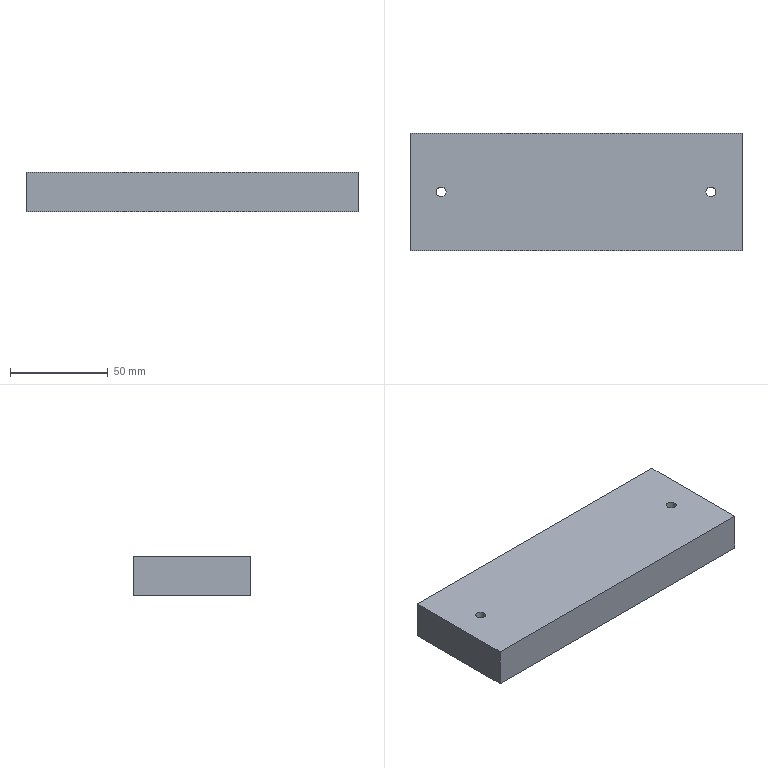CAM job | NX | 3-axis milling, drilling | part box 170 x 60 x 20 mm
Tools:
number,name,description,diameter,corner_radius,flute_length,length,flutes
15,D63,Milling Tool-5 Parameters,63.0,0.0,20.0,20.0,2
10,D12C,Milling Tool-5 Parameters,12.0,0.0,30.0,60.0,2
2,D8,Milling Tool-5 Parameters,8.0,0.0,20.0,50.0,2
3,D6,Milling Tool-5 Parameters,6.0,0.0,15.0,30.0,2
11,D6F,Milling Tool-5 Parameters,6.0,0.0,15.0,30.0,2
4,D4,Milling Tool-5 Parameters,4.0,0.0,10.0,30.0,2
12,D4F,Milling Tool-5 Parameters,4.0,0.0,10.0,25.0,2
5,D3,Milling Tool-5 Parameters,3.0,0.0,10.0,25.0,2
13,D3F,Milling Tool-5 Parameters,3.0,0.0,10.0,25.0,2
6,D2,Milling Tool-5 Parameters,2.0,0.0,5.0,10.0,2
7,D1,Milling Tool-5 Parameters,1.0,0.0,3.0,5.0,2
7,D4R0.5,Milling Tool-5 Parameters,4.0,0.5,10.0,30.0,2
7,D3R0.5,Milling Tool-5 Parameters,3.0,0.5,10.0,30.0,2
20,R1,Milling Tool-Ball Mill,2.0,1.0,5.0,10.0,2
9,D4V45,Milling Tool-5 Parameters,4.0,0.0,10.0,30.0,2
9,D6V45,Milling Tool-5 Parameters,6.0,0.0,10.0,30.0,2
18,ZD5.2,Drilling Tool,5.2,0.0,30.0,50.0,2
19,ZD5,Drilling Tool,5.0,0.0,30.0,35.0,2
12,ZD4.2,Drilling Tool,4.2,0.0,30.0,50.0,2
13,ZD3.3,Drilling Tool,3.3,0.0,30.0,50.0,2
21,ZD3,Drilling Tool,3.0,0.0,30.0,50.0,2
20,ZD1.2,Drilling Tool,1.2,0.0,30.0,50.0,2
20,D4.8-M6X1,Thread Mill,4.8,0.0,0.1,15.0,1
23,CT6,Centerdrill,6.0,0.0,0.0,50.0,2
Operations:
program,operation,operation_type,tool,method,geometry_group,spindle_rpm,surface_speed,feed_per_tooth,feed_cut,feed_plunge,cut_length_mm,path_length_mm,cut_time_min,machine_time_min
GP3-1-1,SPOT_DRILL._COPY,Operation,CT6,METHOD,W-1,3000.0,56.0,0.1667,1000.0,80.0,15.0,248.278,0.015,0.0383
GP3-1-1,DRILL._COPY,Operation,ZD5.2,METHOD,W-1,800.0,13.0,0.0625,100.0,80.0,49.124,257.253,0.4912,0.5121
GP3-1-1,DRILL._COPY_COPY,Operation,ZD3,METHOD,W-1,800.0,13.0,0.0625,100.0,80.0,24.0,202.472,0.24,0.2578
GP3-1-1,ZLEVEL_ROUGH._COPY,ZLevelMilling,D3,METHOD,W-1,5000.0,47.0,0.2,2000.0,80.0,623.78,850.615,0.3157,0.3383
GP3-1-1,ZLEVEL_FINISH._COPY,ZLevelMilling,D3R0.5,METHOD,W-1,8000.0,251.0,0.1875,3000.0,80.0,1064.424,1331.397,0.3554,0.3962
GP3-1-1,2D_CHAMFER._COPY,PlanarMilling,D6V45,METHOD,W-1,5000.0,125.0,0.1,1000.0,50.0,468.51,491.51,0.4701,0.4724
GP3-1-1,2D_CHAMFER._COPY_COPY,PlanarMilling,D6V45,METHOD,W-1,5000.0,125.0,0.1,1000.0,50.0,57.322,240.822,0.0635,0.0818
GP3-1-1,THREAD_MILL._COPY,ThreadMilling,D4.8-M6X1,METHOD,W-1,6000.0,90.0,0.3333,2000.0,50.0,241.604,519.604,0.1227,0.1505
GP3-1-2,3D_ROUGH_COPY,CavityMilling,D12C,METHOD,W-2,8000.0,301.0,0.375,6000.0,80.0,684.95,1013.851,0.1171,0.1657
GP3-1-2,ADAPTIVE_MILL_COPY,CavityMilling,D12C,METHOD,W-2,8000.0,301.0,0.25,4000.0,80.0,1559.391,1648.345,0.39,0.3989
GP3-1-2,3D_ROUGH_COPY_1,CavityMilling,D12C,METHOD,W-2,8000.0,301.0,0.375,6000.0,80.0,5873.405,7165.659,1.003,1.153
GP3-1-2,SPOT_DRILL_COPY,Operation,D6V45,METHOD,W-2,3000.0,56.0,0.25,1500.0,80.0,16.0,152.352,0.0107,0.0243
GP3-1-2,SPOT_DRILL_COPY_COPY,Operation,D6V45,METHOD,W-2,3000.0,56.0,0.25,1500.0,80.0,12.0,307.477,0.008,0.0375
GP3-1-2,SPOT_DRILL_COPY_COPY_COPY,Operation,D6V45,METHOD,W-2,3000.0,56.0,0.25,1500.0,80.0,8.0,131.034,0.0053,0.0176
GP3-1-2,DRILL_COPY,Operation,ZD5,METHOD,W-2,2000.0,32.0,0.075,300.0,80.0,45.004,182.968,0.15,0.1638
GP3-1-2,DRILL_COPY_COPY,Operation,ZD4.2,METHOD,W-2,2000.0,32.0,0.075,300.0,80.0,44.524,148.022,0.1484,0.1588
GP3-1-2,DRILL_COPY_1,Operation,ZD3.3,METHOD,W-2,2000.0,32.0,0.075,300.0,80.0,42.4,323.329,0.1413,0.1694
GP3-1-2,DRILL_COPY_1_COPY_1,Operation,ZD3.3,METHOD,W-2,2000.0,32.0,0.075,300.0,80.0,16.8,141.599,0.056,0.0685
GP3-1-2,DRILL_COPY_1_COPY,Operation,ZD1.2,METHOD,W-2,2000.0,7.0,0.025,100.0,80.0,120.484,361.32,1.205,1.229
GP3-1-2,3D_ROUGH_COPY_1_COPY,CavityMilling,D6,METHOD,W-2,10000.0,188.0,0.25,5000.0,80.0,4024.878,6570.952,0.8573,1.196
GP3-1-2,2D_LAYER_FINISH_MIDENTRY_COPY,PlanarMilling,D6,METHOD,W-2,10000.0,314.0,0.15,3000.0,50.0,199.534,676.857,0.0691,0.13
GP3-1-2,2D_HYBRID_MILL_COPY,PlanarMilling,D6,METHOD,W-2,10000.0,314.0,0.25,5000.0,80.0,991.46,1193.643,0.2003,0.2265
GP3-1-2,HOLE_MILL_COPY,CylinderMilling,D6,METHOD,W-2,10000.0,251.0,0.25,5000.0,80.0,372.596,612.336,0.0753,0.1029
GP3-1-2,2D_PLANAR_FINISH_COPY,FaceMilling,D63,METHOD,W-2,5000.0,989.0,0.15,1500.0,80.0,143.2,224.006,0.0965,0.1046
GP3-1-2,2D_PLANAR_FINISH_COPY_1,FaceMilling,D6F,METHOD,W-2,10000.0,314.0,0.1,2000.0,80.0,131.641,264.818,0.0667,0.0824
GP3-1-2,2D_PLANAR_FINISH_COPY_1_COPY,FaceMilling,D6F,METHOD,W-2,10000.0,314.0,0.1,2000.0,80.0,131.641,264.818,0.0667,0.0824
GP3-1-2,2D_PLANAR_FOLLOW_FINISH_COPY,FaceMilling,D6F,METHOD,W-2,10000.0,314.0,0.1,2000.0,80.0,88.555,330.693,0.0448,0.069
GP3-1-2,BOTTOM_ZIGZAG_FINISH_COPY,FaceMilling,D6F,METHOD,W-2,10000.0,314.0,0.1,2000.0,80.0,469.845,918.349,0.2366,0.2864
GP3-1-2,BOTTOM_ZIGZAG_FINISH_COPY_COPY,FaceMilling,D6F,METHOD,W-2,10000.0,314.0,0.1,2000.0,80.0,467.953,914.7,0.2356,0.2875
GP3-1-2,2D_LAYER_FINISH_CORNER_COPY,PlanarMilling,D6F,METHOD,W-2,10000.0,314.0,0.075,1500.0,50.0,459.076,552.421,0.3085,0.3178
GP3-1-2,2D_LAYER_FINISH_CORNER_COPY_COPY,PlanarMilling,D6F,METHOD,W-2,10000.0,314.0,0.075,1500.0,50.0,60.273,284.35,0.0429,0.0653
GP3-1-2,2D_LAYER_FINISH_CORNER_COPY_COPY_1,PlanarMilling,D6F,METHOD,W-2,10000.0,314.0,0.075,1500.0,50.0,510.334,609.302,0.3427,0.3526
GP3-1-2,2D_LAYER_FINISH_MIDENTRY_COPY_COPY,PlanarMilling,D6F,METHOD,W-2,10000.0,314.0,0.075,1500.0,50.0,408.754,887.101,0.2827,0.3437
GP3-1-2,2D_LAYER_FINISH_CORNER_COPY_COPY_COPY,PlanarMilling,D6F,METHOD,W-2,10000.0,314.0,0.075,1500.0,50.0,627.953,733.315,0.4211,0.4317
GP3-1-2,2D_PLANAR_BOTTOM_SIDE_FINISH_COPY,FaceMilling,D6F,METHOD,W-2,10000.0,314.0,0.075,1500.0,80.0,180.859,685.942,0.1236,0.1741
GP3-1-2,HOLE_MILL_COPY_1,CylinderMilling,D4,METHOD,W-2,10000.0,125.0,0.1,2000.0,80.0,950.58,1410.071,0.4764,0.5368
GP3-1-2,ONEPASS_CORNER_CLEAN_COPY,ZLevelMilling,D4,METHOD,W-2,10000.0,125.0,0.1,2000.0,80.0,410.036,978.176,0.2065,0.2634
GP3-1-2,3D_ZLEVEL_ROUGH_COPY,ZLevelMilling,D4,METHOD,W-2,10000.0,125.0,0.1,2000.0,80.0,3034.754,3575.086,1.529,1.583
GP3-1-2,3D_ZLEVEL_FINISH_COPY,ZLevelMilling,D4R0.5,METHOD,W-2,10000.0,125.0,0.15,3000.0,80.0,2041.47,2556.017,0.681,0.7325
GP3-1-2,2D_PLANAR_BOTTOM_SIDE_FINISH_COPY_1,FaceMilling,D4F,METHOD,W-2,10000.0,125.0,0.025,500.0,80.0,61.474,1059.284,0.1289,0.2287
GP3-1-2,2D_LAYER_FINISH_CORNER_COPY_COPY_1_COPY,PlanarMilling,D4F,METHOD,W-2,10000.0,125.0,0.025,500.0,50.0,58.266,645.108,0.1374,0.1961
GP3-1-2,2D_PLANAR_BOTTOM_SIDE_FINISH_COPY_1_COPY,FaceMilling,D4F,METHOD,W-2,10000.0,125.0,0.025,500.0,80.0,62.895,694.212,0.1291,0.1923
GP3-1-2,2D_LAYER_FINISH_CORNER_COPY_COPY_1_COPY_COPY_1,PlanarMilling,D4F,METHOD,W-2,10000.0,125.0,0.025,500.0,50.0,24.837,366.346,0.0583,0.0925
GP3-1-2,2D_LAYER_FINISH_CORNER_COPY_COPY_1_COPY_COPY_1_COPY,PlanarMilling,D3F,METHOD,W-2,13263.0,125.0,0.0188,500.0,50.0,30.149,337.774,0.073,0.1038
GP3-1-2,3D_ZLEVEL_ROUGH_COPY_1,ZLevelMilling,D2,METHOD,W-2,10000.0,62.0,0.1,2000.0,80.0,428.56,850.715,0.2241,0.2663
GP3-1-2,2D_PLANAR_BOTTOM_SIDE_FINISH_COPY_COPY,FaceMilling,D2,METHOD,W-2,10000.0,62.0,0.01,200.0,80.0,166.941,628.781,0.8415,0.8877
GP3-1-2,HOLE_MILL_COPY_2,CylinderMilling,D1,METHOD,W-2,10000.0,31.0,0.1,2000.0,80.0,141.27,381.486,0.0709,0.0991
GP3-1-2,HOLE_MILL_COPY_2_COPY,CylinderMilling,D1,METHOD,W-2,10000.0,31.0,0.1,2000.0,80.0,187.035,427.651,0.0939,0.1221
GP3-1-2,2D_CHAMFER_COPY,PlanarMilling,D6V45,METHOD,W-2,12000.0,150.0,0.0833,2000.0,50.0,211.533,290.897,0.1065,0.1145
GP3-1-2,2D_CHAMFER_COPY_COPY,PlanarMilling,D6V45,METHOD,W-2,12000.0,150.0,0.0833,2000.0,50.0,109.012,478.172,0.0576,0.0945
GP3-1-2,SPOT_DRILL_COPY_COPY_1,Operation,D6V45,METHOD,W-2,3000.0,56.0,0.25,1500.0,80.0,16.2,153.532,0.0108,0.0245
GP3-1-2,2D_CHAMFER_COPY_COPY_1,PlanarMilling,D6V45,METHOD,W-2,12000.0,150.0,0.0833,2000.0,50.0,135.959,814.83,0.0711,0.139
GP3-1-2,2D_CHAMFER_COPY_COPY_1_COPY,PlanarMilling,D6V45,METHOD,W-2,12000.0,150.0,0.0833,2000.0,50.0,70.145,730.545,0.0382,0.1042
GP3-1-2,2D_CHAMFER_COPY_COPY_1_COPY_COPY,PlanarMilling,D6V45,METHOD,W-2,12000.0,150.0,0.0833,2000.0,50.0,17.536,138.936,0.0095,0.0217
GP3-1-2,2D_CHAMFER_NO_LEAD_COPY,PlanarMilling,D6V45,METHOD,W-2,12000.0,150.0,0.0833,2000.0,50.0,23.624,146.024,0.0118,0.0241
GP3-1-2,2D_CHAMFER_NO_LEAD_COPY_COPY,PlanarMilling,D6V45,METHOD,W-2,12000.0,150.0,0.0833,2000.0,50.0,3.783,130.743,0.0019,0.0146
GP3-1-2,2D_CHAMFER_NO_LEAD_COPY_COPY_COPY,PlanarMilling,D6V45,METHOD,W-2,12000.0,150.0,0.0833,2000.0,50.0,184.759,1058.577,0.0924,0.1798
GP3-1-3,3D_ROUGH_COPY_COPY,CavityMilling,D12C,METHOD,W-3,8000.0,301.0,0.375,6000.0,80.0,2657.234,3228.722,0.4535,0.5425
GP3-1-3,3D_ROUGH_COPY_COPY_COPY,CavityMilling,D12C,METHOD,W-3,8000.0,301.0,0.375,6000.0,80.0,305.419,324.969,0.0514,0.0534
GP3-1-3,3D_ROUGH_COPY_1_COPY_COPY,CavityMilling,D8,METHOD,W-3,10000.0,188.0,0.25,5000.0,80.0,41.837,220.538,0.0089,0.0267
GP3-1-3,3D_ZLEVEL_ROUGH_COPY_2,ZLevelMilling,D8,METHOD,W-3,10000.0,251.0,0.3,6000.0,80.0,5112.692,5183.583,0.8541,0.8625
GP3-1-3,2D_PLANAR_FINISH_COPY_COPY,FaceMilling,D63,METHOD,W-3,5000.0,989.0,0.15,1500.0,80.0,170.6,190.4,0.1148,0.1168
GP3-1-3,BOTTOM_ZIGZAG_FINISH_COPY_COPY_1,FaceMilling,D6F,METHOD,W-3,10000.0,314.0,0.1,2000.0,80.0,776.89,797.49,0.3889,0.391
GP3-1-3,2D_PLANAR_BOTTOM_SIDE_FINISH_COPY_COPY_1,FaceMilling,D6F,METHOD,W-3,10000.0,314.0,0.075,1500.0,80.0,408.46,429.06,0.273,0.275
GP3-1-3,HOLE_MILL_COPY_COPY,CylinderMilling,D4,METHOD,W-3,10000.0,251.0,0.25,5000.0,80.0,207.708,536.508,0.0418,0.0892
GP3-1-3,3D_ROUGH_COPY_1_COPY_COPY_COPY,CavityMilling,D4,METHOD,W-3,10000.0,125.0,0.1,2000.0,80.0,87.049,376.626,0.0472,0.0761
GP3-1-3,3D_ROUGH_COPY_1_COPY_COPY_COPY_COPY,CavityMilling,D4,METHOD,W-3,10000.0,125.0,0.1,2000.0,80.0,3919.109,5650.118,2.047,2.311
GP3-1-3,3D_ROUGH_COPY_1_COPY_COPY_COPY_COPY_COPY,CavityMilling,D3,METHOD,W-3,10000.0,125.0,0.1,2000.0,80.0,3222.457,4459.841,1.677,1.858
GP3-1-3,3D_HYBRID_COPY,ZLevelMilling,R1,METHOD,W-3,10000.0,62.0,0.1,2000.0,80.0,1344.942,1408.336,0.6813,0.6883
GP3-1-3,3D_HYBRID_COPY_COPY,ZLevelMilling,R1,METHOD,W-3,10000.0,62.0,0.1,2000.0,80.0,557.649,616.111,0.2843,0.2908
GP3-1-3,SURFACE_FINISH_COPY,SurfaceContour,R1,METHOD,W-3,19894.0,125.0,0.0503,2000.0,80.0,648.536,769.807,0.3322,0.3483
GP3-1-3,2D_PLANAR_BOTTOM_SIDE_FINISH_COPY_2,FaceMilling,D4F,METHOD,W-3,5000.0,62.0,0.05,500.0,80.0,71.796,426.606,0.1501,0.1855
GP3-1-3,BOTTOM_ZIGZAG_FINISH_COPY_COPY_1_COPY,FaceMilling,D3F,METHOD,W-3,10000.0,314.0,0.1,2000.0,80.0,421.536,533.9,0.2112,0.2224
GP3-1-3,2D_LAYER_FINISH_MIDENTRY_COPY_1,PlanarMilling,D3F,METHOD,W-3,10000.0,94.0,0.05,1000.0,50.0,675.841,842.696,0.6838,0.7032
GP3-1-3,3D_ROUGH_COPY_1_COPY_COPY_COPY_COPY_1,CavityMilling,D2,METHOD,W-3,10000.0,125.0,0.1,2000.0,80.0,107.031,358.848,0.0548,0.083
GP3-1-3,HOLE_MILL_COPY_2_COPY_1,CylinderMilling,D1,METHOD,W-3,10000.0,31.0,0.1,2000.0,80.0,45.761,200.981,0.023,0.0438
GP3-1-3,HOLE_MILL_COPY_2_COPY_1_COPY,CylinderMilling,D1,METHOD,W-3,10000.0,31.0,0.1,2000.0,80.0,70.103,225.523,0.0352,0.056
GP3-1-3,2D_CHAMFER_COPY_COPY_2,PlanarMilling,D4V45,METHOD,W-3,12000.0,150.0,0.0833,2000.0,50.0,294.904,316.904,0.148,0.1502
GP3-1-3,2D_CHAMFER_COPY_COPY_2_COPY,PlanarMilling,D4V45,METHOD,W-3,12000.0,150.0,0.0833,2000.0,50.0,78.313,427.913,0.0422,0.0772
GP3-1-3,2D_CHAMFER_COPY_COPY_2_COPY_COPY,PlanarMilling,D4V45,METHOD,W-3,12000.0,150.0,0.0833,2000.0,50.0,17.48,391.08,0.0103,0.0476
GP3-1-3,2D_CHAMFER_COPY_COPY_2_COPY_COPY_COPY,PlanarMilling,D4V45,METHOD,W-3,12000.0,150.0,0.0833,2000.0,50.0,222.597,242.997,0.1118,0.1139
GP3-1-3,2D_CHAMFER_COPY_COPY_2_COPY_COPY_COPY_COPY,PlanarMilling,D4V45,METHOD,W-3,12000.0,150.0,0.0833,2000.0,50.0,12.91,169.11,0.0075,0.0231
GP3-1-3,2D_CHAMFER_COPY_COPY_2_COPY_COPY_COPY_COPY_COPY,PlanarMilling,D4V45,METHOD,W-3,12000.0,150.0,0.0833,2000.0,50.0,174.014,253.468,0.088,0.096